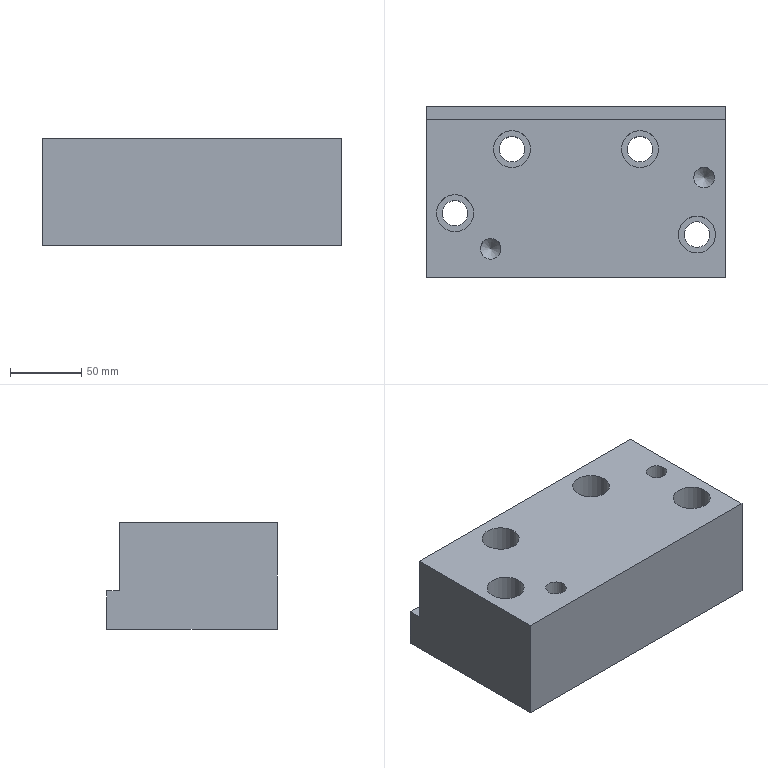Part | STEP file | lll_id550_x_t | 1 solid | 28 faces | box 210 x 120 x 75 mm | volume 1667876 mm3 | plane 12 | cylinder 12 | cone 4 | commonest cylinder face diameters 18.009 x4 26.008 x4 8.506 x2 14.506 x2
STEP:
#1=CARTESIAN_POINT('',(2294.339,-512.386,-95.));
#2=VERTEX_POINT('',#1);
#3=CARTESIAN_POINT('',(2504.339,-512.386,-95.));
#4=VERTEX_POINT('',#3);
#5=CARTESIAN_POINT('',(2648.249,-512.386,-95.));
#6=DIRECTION('',(1.,0.,0.));
#7=VECTOR('',#6,1.);
#8=LINE('',#5,#7);
#9=EDGE_CURVE('',#2,#4,#8,.T.);
#10=ORIENTED_EDGE('',*,*,#9,.T.);
#11=CARTESIAN_POINT('',(2504.339,-512.386,-20.));
#12=VERTEX_POINT('',#11);
#13=CARTESIAN_POINT('',(2504.339,-512.386,-60.));
#14=DIRECTION('',(0.,0.,-1.));
#15=VECTOR('',#14,1.);
#16=LINE('',#13,#15);
#17=EDGE_CURVE('',#12,#4,#16,.T.);
#18=ORIENTED_EDGE('',*,*,#17,.F.);
#19=CARTESIAN_POINT('',(2294.339,-512.386,-20.));
#20=VERTEX_POINT('',#19);
#21=CARTESIAN_POINT('',(-2203.001,-512.386,-20.));
#22=DIRECTION('',(-1.,0.,0.));
#23=VECTOR('',#22,1.);
#24=LINE('',#21,#23);
#25=EDGE_CURVE('',#12,#20,#24,.T.);
#26=ORIENTED_EDGE('',*,*,#25,.T.);
#27=CARTESIAN_POINT('',(2294.339,-512.386,72.5));
#28=DIRECTION('',(0.,0.,-1.));
#29=VECTOR('',#28,1.);
#30=LINE('',#27,#29);
#31=EDGE_CURVE('',#20,#2,#30,.T.);
#32=ORIENTED_EDGE('',*,*,#31,.T.);
#33=EDGE_LOOP('',(#10,#18,#26,#32));
#34=FACE_OUTER_BOUND('',#33,.T.);
#35=CARTESIAN_POINT('',(-2203.001,-512.386,-650.));
#36=DIRECTION('',(0.,1.,0.));
#37=DIRECTION('',(0.,0.,1.));
#38=AXIS2_PLACEMENT_3D('',#35,#36,#37);
#39=PLANE('',#38);
#40=ADVANCED_FACE('',(#34),#39,.F.);
#41=CARTESIAN_POINT('',(2493.344,-482.386,-95.));
#42=VERTEX_POINT('',#41);
#43=CARTESIAN_POINT('',(2484.339,-482.386,-95.));
#44=DIRECTION('',(0.,0.,1.));
#45=DIRECTION('',(1.,0.,0.));
#46=AXIS2_PLACEMENT_3D('',#43,#44,#45);
#47=CIRCLE('',#46,9.005);
#48=EDGE_CURVE('',#42,#42,#47,.T.);
#49=ORIENTED_EDGE('',*,*,#48,.T.);
#50=EDGE_LOOP('',(#49));
#51=FACE_BOUND('',#50,.T.);
#52=CARTESIAN_POINT('',(2323.344,-467.386,-95.));
#53=VERTEX_POINT('',#52);
#54=CARTESIAN_POINT('',(2314.339,-467.386,-95.));
#55=DIRECTION('',(0.,0.,1.));
#56=DIRECTION('',(1.,0.,0.));
#57=AXIS2_PLACEMENT_3D('',#54,#55,#56);
#58=CIRCLE('',#57,9.005);
#59=EDGE_CURVE('',#53,#53,#58,.T.);
#60=ORIENTED_EDGE('',*,*,#59,.T.);
#61=EDGE_LOOP('',(#60));
#62=FACE_BOUND('',#61,.T.);
#63=CARTESIAN_POINT('',(2453.344,-422.386,-95.));
#64=VERTEX_POINT('',#63);
#65=CARTESIAN_POINT('',(2444.339,-422.386,-95.));
#66=DIRECTION('',(0.,0.,1.));
#67=DIRECTION('',(1.,0.,0.));
#68=AXIS2_PLACEMENT_3D('',#65,#66,#67);
#69=CIRCLE('',#68,9.005);
#70=EDGE_CURVE('',#64,#64,#69,.T.);
#71=ORIENTED_EDGE('',*,*,#70,.T.);
#72=EDGE_LOOP('',(#71));
#73=FACE_BOUND('',#72,.T.);
#74=CARTESIAN_POINT('',(2363.344,-422.386,-95.));
#75=VERTEX_POINT('',#74);
#76=CARTESIAN_POINT('',(2354.339,-422.386,-95.));
#77=DIRECTION('',(0.,0.,1.));
#78=DIRECTION('',(1.,0.,0.));
#79=AXIS2_PLACEMENT_3D('',#76,#77,#78);
#80=CIRCLE('',#79,9.005);
#81=EDGE_CURVE('',#75,#75,#80,.T.);
#82=ORIENTED_EDGE('',*,*,#81,.T.);
#83=EDGE_LOOP('',(#82));
#84=FACE_BOUND('',#83,.T.);
#85=ORIENTED_EDGE('',*,*,#9,.F.);
#86=CARTESIAN_POINT('',(2294.339,-392.386,-95.));
#87=VERTEX_POINT('',#86);
#88=CARTESIAN_POINT('',(2294.339,-442.386,-95.));
#89=DIRECTION('',(0.,1.,0.));
#90=VECTOR('',#89,1.);
#91=LINE('',#88,#90);
#92=EDGE_CURVE('',#2,#87,#91,.T.);
#93=ORIENTED_EDGE('',*,*,#92,.T.);
#94=CARTESIAN_POINT('',(2504.339,-392.386,-95.));
#95=VERTEX_POINT('',#94);
#96=CARTESIAN_POINT('',(-2203.001,-392.386,-95.));
#97=DIRECTION('',(1.,0.,0.));
#98=VECTOR('',#97,1.);
#99=LINE('',#96,#98);
#100=EDGE_CURVE('',#87,#95,#99,.T.);
#101=ORIENTED_EDGE('',*,*,#100,.T.);
#102=CARTESIAN_POINT('',(2504.339,-268.547,-95.));
#103=DIRECTION('',(0.,-1.,0.));
#104=VECTOR('',#103,1.);
#105=LINE('',#102,#104);
#106=EDGE_CURVE('',#95,#4,#105,.T.);
#107=ORIENTED_EDGE('',*,*,#106,.T.);
#108=EDGE_LOOP('',(#85,#93,#101,#107));
#109=FACE_BOUND('',#108,.T.);
#110=CARTESIAN_POINT('',(2648.249,-268.547,-95.));
#111=DIRECTION('',(0.,0.,-1.));
#112=DIRECTION('',(1.,0.,0.));
#113=AXIS2_PLACEMENT_3D('',#110,#111,#112);
#114=PLANE('',#113);
#115=ADVANCED_FACE('',(#51,#62,#73,#84,#109),#114,.T.);
#116=CARTESIAN_POINT('',(2504.339,-401.386,-20.));
#117=VERTEX_POINT('',#116);
#118=CARTESIAN_POINT('',(2504.339,-417.386,-20.));
#119=DIRECTION('',(0.,1.,0.));
#120=VECTOR('',#119,1.);
#121=LINE('',#118,#120);
#122=EDGE_CURVE('',#12,#117,#121,.T.);
#123=ORIENTED_EDGE('',*,*,#122,.T.);
#124=CARTESIAN_POINT('',(2294.339,-401.386,-20.));
#125=VERTEX_POINT('',#124);
#126=CARTESIAN_POINT('',(-2203.001,-401.386,-20.));
#127=DIRECTION('',(1.,0.,0.));
#128=VECTOR('',#127,1.);
#129=LINE('',#126,#128);
#130=EDGE_CURVE('',#125,#117,#129,.T.);
#131=ORIENTED_EDGE('',*,*,#130,.F.);
#132=CARTESIAN_POINT('',(2294.339,-417.386,-20.));
#133=DIRECTION('',(0.,-1.,0.));
#134=VECTOR('',#133,1.);
#135=LINE('',#132,#134);
#136=EDGE_CURVE('',#125,#20,#135,.T.);
#137=ORIENTED_EDGE('',*,*,#136,.T.);
#138=ORIENTED_EDGE('',*,*,#25,.F.);
#139=EDGE_LOOP('',(#123,#131,#137,#138));
#140=FACE_BOUND('',#139,.T.);
#141=CARTESIAN_POINT('',(2346.592,-492.386,-20.));
#142=VERTEX_POINT('',#141);
#143=CARTESIAN_POINT('',(2339.339,-492.386,-20.));
#144=DIRECTION('',(0.,0.,1.));
#145=DIRECTION('',(1.,0.,0.));
#146=AXIS2_PLACEMENT_3D('',#143,#144,#145);
#147=CIRCLE('',#146,7.253);
#148=EDGE_CURVE('',#142,#142,#147,.T.);
#149=ORIENTED_EDGE('',*,*,#148,.F.);
#150=EDGE_LOOP('',(#149));
#151=FACE_BOUND('',#150,.T.);
#152=CARTESIAN_POINT('',(2496.592,-442.386,-20.));
#153=VERTEX_POINT('',#152);
#154=CARTESIAN_POINT('',(2489.339,-442.386,-20.));
#155=DIRECTION('',(0.,0.,1.));
#156=DIRECTION('',(1.,0.,0.));
#157=AXIS2_PLACEMENT_3D('',#154,#155,#156);
#158=CIRCLE('',#157,7.253);
#159=EDGE_CURVE('',#153,#153,#158,.T.);
#160=ORIENTED_EDGE('',*,*,#159,.F.);
#161=EDGE_LOOP('',(#160));
#162=FACE_BOUND('',#161,.T.);
#163=CARTESIAN_POINT('',(2471.335,-482.386,-20.));
#164=VERTEX_POINT('',#163);
#165=CARTESIAN_POINT('',(2484.339,-482.386,-20.));
#166=DIRECTION('',(0.,0.,1.));
#167=DIRECTION('',(-1.,0.,0.));
#168=AXIS2_PLACEMENT_3D('',#165,#166,#167);
#169=CIRCLE('',#168,13.004);
#170=EDGE_CURVE('',#164,#164,#169,.T.);
#171=ORIENTED_EDGE('',*,*,#170,.F.);
#172=EDGE_LOOP('',(#171));
#173=FACE_BOUND('',#172,.T.);
#174=CARTESIAN_POINT('',(2301.335,-467.386,-20.));
#175=VERTEX_POINT('',#174);
#176=CARTESIAN_POINT('',(2314.339,-467.386,-20.));
#177=DIRECTION('',(0.,0.,1.));
#178=DIRECTION('',(-1.,0.,0.));
#179=AXIS2_PLACEMENT_3D('',#176,#177,#178);
#180=CIRCLE('',#179,13.004);
#181=EDGE_CURVE('',#175,#175,#180,.T.);
#182=ORIENTED_EDGE('',*,*,#181,.F.);
#183=EDGE_LOOP('',(#182));
#184=FACE_BOUND('',#183,.T.);
#185=CARTESIAN_POINT('',(2431.335,-422.386,-20.));
#186=VERTEX_POINT('',#185);
#187=CARTESIAN_POINT('',(2444.339,-422.386,-20.));
#188=DIRECTION('',(0.,0.,1.));
#189=DIRECTION('',(-1.,0.,0.));
#190=AXIS2_PLACEMENT_3D('',#187,#188,#189);
#191=CIRCLE('',#190,13.004);
#192=EDGE_CURVE('',#186,#186,#191,.T.);
#193=ORIENTED_EDGE('',*,*,#192,.F.);
#194=EDGE_LOOP('',(#193));
#195=FACE_BOUND('',#194,.T.);
#196=CARTESIAN_POINT('',(2367.343,-422.386,-20.));
#197=VERTEX_POINT('',#196);
#198=CARTESIAN_POINT('',(2354.339,-422.386,-20.));
#199=DIRECTION('',(0.,0.,-1.));
#200=DIRECTION('',(1.,0.,0.));
#201=AXIS2_PLACEMENT_3D('',#198,#199,#200);
#202=CIRCLE('',#201,13.004);
#203=EDGE_CURVE('',#197,#197,#202,.T.);
#204=ORIENTED_EDGE('',*,*,#203,.T.);
#205=EDGE_LOOP('',(#204));
#206=FACE_BOUND('',#205,.T.);
#207=CARTESIAN_POINT('',(2402.588,-417.386,-20.));
#208=DIRECTION('',(0.,0.,-1.));
#209=DIRECTION('',(1.,0.,0.));
#210=AXIS2_PLACEMENT_3D('',#207,#208,#209);
#211=PLANE('',#210);
#212=ADVANCED_FACE('',(#140,#151,#162,#173,#184,#195,#206),#211,.F.);
#213=CARTESIAN_POINT('',(2470.086,-401.386,-44.));
#214=VERTEX_POINT('',#213);
#215=CARTESIAN_POINT('',(2474.339,-401.386,-44.));
#216=DIRECTION('',(0.,1.,0.));
#217=DIRECTION('',(-1.,0.,0.));
#218=AXIS2_PLACEMENT_3D('',#215,#216,#217);
#219=CIRCLE('',#218,4.253);
#220=EDGE_CURVE('',#214,#214,#219,.T.);
#221=ORIENTED_EDGE('',*,*,#220,.F.);
#222=EDGE_LOOP('',(#221));
#223=FACE_BOUND('',#222,.T.);
#224=CARTESIAN_POINT('',(2294.339,-401.386,-68.));
#225=VERTEX_POINT('',#224);
#226=CARTESIAN_POINT('',(2504.339,-401.386,-68.));
#227=VERTEX_POINT('',#226);
#228=CARTESIAN_POINT('',(2399.339,-401.386,-68.));
#229=DIRECTION('',(1.,0.,0.));
#230=VECTOR('',#229,1.);
#231=LINE('',#228,#230);
#232=EDGE_CURVE('',#225,#227,#231,.T.);
#233=ORIENTED_EDGE('',*,*,#232,.F.);
#234=CARTESIAN_POINT('',(2294.339,-401.386,-650.));
#235=DIRECTION('',(0.,0.,-1.));
#236=VECTOR('',#235,1.);
#237=LINE('',#234,#236);
#238=EDGE_CURVE('',#125,#225,#237,.T.);
#239=ORIENTED_EDGE('',*,*,#238,.F.);
#240=ORIENTED_EDGE('',*,*,#130,.T.);
#241=CARTESIAN_POINT('',(2504.339,-401.386,-60.));
#242=DIRECTION('',(0.,0.,1.));
#243=VECTOR('',#242,1.);
#244=LINE('',#241,#243);
#245=EDGE_CURVE('',#227,#117,#244,.T.);
#246=ORIENTED_EDGE('',*,*,#245,.F.);
#247=EDGE_LOOP('',(#233,#239,#240,#246));
#248=FACE_BOUND('',#247,.T.);
#249=CARTESIAN_POINT('',(2320.086,-401.386,-44.));
#250=VERTEX_POINT('',#249);
#251=CARTESIAN_POINT('',(2324.339,-401.386,-44.));
#252=DIRECTION('',(0.,1.,0.));
#253=DIRECTION('',(-1.,0.,0.));
#254=AXIS2_PLACEMENT_3D('',#251,#252,#253);
#255=CIRCLE('',#254,4.253);
#256=EDGE_CURVE('',#250,#250,#255,.T.);
#257=ORIENTED_EDGE('',*,*,#256,.F.);
#258=EDGE_LOOP('',(#257));
#259=FACE_BOUND('',#258,.T.);
#260=CARTESIAN_POINT('',(-2203.001,-401.386,-650.));
#261=DIRECTION('',(0.,1.,0.));
#262=DIRECTION('',(0.,0.,1.));
#263=AXIS2_PLACEMENT_3D('',#260,#261,#262);
#264=PLANE('',#263);
#265=ADVANCED_FACE('',(#223,#248,#259),#264,.T.);
#266=CARTESIAN_POINT('',(2294.339,-392.386,-68.));
#267=VERTEX_POINT('',#266);
#268=CARTESIAN_POINT('',(2294.339,-392.386,72.5));
#269=DIRECTION('',(0.,0.,-1.));
#270=VECTOR('',#269,1.);
#271=LINE('',#268,#270);
#272=EDGE_CURVE('',#267,#87,#271,.T.);
#273=ORIENTED_EDGE('',*,*,#272,.T.);
#274=ORIENTED_EDGE('',*,*,#92,.F.);
#275=ORIENTED_EDGE('',*,*,#31,.F.);
#276=ORIENTED_EDGE('',*,*,#136,.F.);
#277=ORIENTED_EDGE('',*,*,#238,.T.);
#278=CARTESIAN_POINT('',(2294.339,-432.386,-68.));
#279=DIRECTION('',(0.,1.,0.));
#280=VECTOR('',#279,1.);
#281=LINE('',#278,#280);
#282=EDGE_CURVE('',#225,#267,#281,.T.);
#283=ORIENTED_EDGE('',*,*,#282,.T.);
#284=EDGE_LOOP('',(#273,#274,#275,#276,#277,#283));
#285=FACE_OUTER_BOUND('',#284,.T.);
#286=CARTESIAN_POINT('',(2294.339,-442.386,72.5));
#287=DIRECTION('',(-1.,0.,0.));
#288=DIRECTION('',(0.,0.,-1.));
#289=AXIS2_PLACEMENT_3D('',#286,#287,#288);
#290=PLANE('',#289);
#291=ADVANCED_FACE('',(#285),#290,.T.);
#292=CARTESIAN_POINT('',(2504.339,-392.386,-68.));
#293=VERTEX_POINT('',#292);
#294=CARTESIAN_POINT('',(2504.339,-392.386,-60.));
#295=DIRECTION('',(0.,0.,1.));
#296=VECTOR('',#295,1.);
#297=LINE('',#294,#296);
#298=EDGE_CURVE('',#95,#293,#297,.T.);
#299=ORIENTED_EDGE('',*,*,#298,.F.);
#300=ORIENTED_EDGE('',*,*,#100,.F.);
#301=ORIENTED_EDGE('',*,*,#272,.F.);
#302=CARTESIAN_POINT('',(-2203.001,-392.386,-68.));
#303=DIRECTION('',(-1.,0.,0.));
#304=VECTOR('',#303,1.);
#305=LINE('',#302,#304);
#306=EDGE_CURVE('',#293,#267,#305,.T.);
#307=ORIENTED_EDGE('',*,*,#306,.F.);
#308=EDGE_LOOP('',(#299,#300,#301,#307));
#309=FACE_OUTER_BOUND('',#308,.T.);
#310=CARTESIAN_POINT('',(-2203.001,-392.386,-650.));
#311=DIRECTION('',(0.,1.,0.));
#312=DIRECTION('',(0.,0.,1.));
#313=AXIS2_PLACEMENT_3D('',#310,#311,#312);
#314=PLANE('',#313);
#315=ADVANCED_FACE('',(#309),#314,.T.);
#316=CARTESIAN_POINT('',(2504.339,-417.386,-68.));
#317=DIRECTION('',(0.,-1.,0.));
#318=VECTOR('',#317,1.);
#319=LINE('',#316,#318);
#320=EDGE_CURVE('',#293,#227,#319,.T.);
#321=ORIENTED_EDGE('',*,*,#320,.T.);
#322=ORIENTED_EDGE('',*,*,#245,.T.);
#323=ORIENTED_EDGE('',*,*,#122,.F.);
#324=ORIENTED_EDGE('',*,*,#17,.T.);
#325=ORIENTED_EDGE('',*,*,#106,.F.);
#326=ORIENTED_EDGE('',*,*,#298,.T.);
#327=EDGE_LOOP('',(#321,#322,#323,#324,#325,#326));
#328=FACE_OUTER_BOUND('',#327,.T.);
#329=CARTESIAN_POINT('',(2504.339,-417.386,-60.));
#330=DIRECTION('',(-1.,0.,0.));
#331=DIRECTION('',(0.,0.,-1.));
#332=AXIS2_PLACEMENT_3D('',#329,#330,#331);
#333=PLANE('',#332);
#334=ADVANCED_FACE('',(#328),#333,.F.);
#335=ORIENTED_EDGE('',*,*,#232,.T.);
#336=ORIENTED_EDGE('',*,*,#320,.F.);
#337=ORIENTED_EDGE('',*,*,#306,.T.);
#338=ORIENTED_EDGE('',*,*,#282,.F.);
#339=EDGE_LOOP('',(#335,#336,#337,#338));
#340=FACE_OUTER_BOUND('',#339,.T.);
#341=CARTESIAN_POINT('',(2399.339,-432.386,-68.));
#342=DIRECTION('',(0.,0.,1.));
#343=DIRECTION('',(-1.,0.,0.));
#344=AXIS2_PLACEMENT_3D('',#341,#342,#343);
#345=PLANE('',#344);
#346=ADVANCED_FACE('',(#340),#345,.T.);
#347=CARTESIAN_POINT('',(2474.339,-432.139,-48.253));
#348=VERTEX_POINT('',#347);
#349=CARTESIAN_POINT('',(2474.339,-432.139,-44.));
#350=DIRECTION('',(0.,1.,0.));
#351=DIRECTION('',(0.,0.,-1.));
#352=AXIS2_PLACEMENT_3D('',#349,#350,#351);
#353=CIRCLE('',#352,4.253);
#354=EDGE_CURVE('',#348,#348,#353,.T.);
#355=ORIENTED_EDGE('',*,*,#354,.F.);
#356=EDGE_LOOP('',(#355));
#357=FACE_BOUND('',#356,.T.);
#358=ORIENTED_EDGE('',*,*,#220,.T.);
#359=EDGE_LOOP('',(#358));
#360=FACE_BOUND('',#359,.T.);
#361=CARTESIAN_POINT('',(2474.339,-401.386,-44.));
#362=DIRECTION('',(0.,-1.,0.));
#363=DIRECTION('',(-1.,0.,0.));
#364=AXIS2_PLACEMENT_3D('',#361,#362,#363);
#365=CYLINDRICAL_SURFACE('',#364,4.253);
#366=ADVANCED_FACE('',(#357,#360),#365,.F.);
#367=CARTESIAN_POINT('',(2474.339,-436.392,-44.));
#368=VERTEX_POINT('',#367);
#369=VERTEX_LOOP('',#368);
#370=FACE_BOUND('',#369,.T.);
#371=ORIENTED_EDGE('',*,*,#354,.T.);
#372=EDGE_LOOP('',(#371));
#373=FACE_BOUND('',#372,.T.);
#374=CARTESIAN_POINT('',(2474.339,-432.139,-44.));
#375=DIRECTION('',(0.,1.,0.));
#376=DIRECTION('',(0.,0.,1.));
#377=AXIS2_PLACEMENT_3D('',#374,#375,#376);
#378=CONICAL_SURFACE('',#377,4.253,45.);
#379=ADVANCED_FACE('',(#370,#373),#378,.F.);
#380=CARTESIAN_POINT('',(2324.339,-432.139,-48.253));
#381=VERTEX_POINT('',#380);
#382=CARTESIAN_POINT('',(2324.339,-432.139,-44.));
#383=DIRECTION('',(0.,1.,0.));
#384=DIRECTION('',(0.,0.,-1.));
#385=AXIS2_PLACEMENT_3D('',#382,#383,#384);
#386=CIRCLE('',#385,4.253);
#387=EDGE_CURVE('',#381,#381,#386,.T.);
#388=ORIENTED_EDGE('',*,*,#387,.F.);
#389=EDGE_LOOP('',(#388));
#390=FACE_BOUND('',#389,.T.);
#391=ORIENTED_EDGE('',*,*,#256,.T.);
#392=EDGE_LOOP('',(#391));
#393=FACE_BOUND('',#392,.T.);
#394=CARTESIAN_POINT('',(2324.339,-401.386,-44.));
#395=DIRECTION('',(0.,-1.,0.));
#396=DIRECTION('',(-1.,0.,0.));
#397=AXIS2_PLACEMENT_3D('',#394,#395,#396);
#398=CYLINDRICAL_SURFACE('',#397,4.253);
#399=ADVANCED_FACE('',(#390,#393),#398,.F.);
#400=CARTESIAN_POINT('',(2324.339,-436.392,-44.));
#401=VERTEX_POINT('',#400);
#402=VERTEX_LOOP('',#401);
#403=FACE_BOUND('',#402,.T.);
#404=ORIENTED_EDGE('',*,*,#387,.T.);
#405=EDGE_LOOP('',(#404));
#406=FACE_BOUND('',#405,.T.);
#407=CARTESIAN_POINT('',(2324.339,-432.139,-44.));
#408=DIRECTION('',(0.,1.,0.));
#409=DIRECTION('',(0.,0.,1.));
#410=AXIS2_PLACEMENT_3D('',#407,#408,#409);
#411=CONICAL_SURFACE('',#410,4.253,45.);
#412=ADVANCED_FACE('',(#403,#406),#411,.F.);
#413=ORIENTED_EDGE('',*,*,#48,.F.);
#414=EDGE_LOOP('',(#413));
#415=FACE_BOUND('',#414,.T.);
#416=CARTESIAN_POINT('',(2493.344,-482.386,-55.));
#417=VERTEX_POINT('',#416);
#418=CARTESIAN_POINT('',(2484.339,-482.386,-55.));
#419=DIRECTION('',(0.,0.,1.));
#420=DIRECTION('',(1.,0.,0.));
#421=AXIS2_PLACEMENT_3D('',#418,#419,#420);
#422=CIRCLE('',#421,9.005);
#423=EDGE_CURVE('',#417,#417,#422,.T.);
#424=ORIENTED_EDGE('',*,*,#423,.T.);
#425=EDGE_LOOP('',(#424));
#426=FACE_BOUND('',#425,.T.);
#427=CARTESIAN_POINT('',(2484.339,-482.386,-18.));
#428=DIRECTION('',(0.,0.,-1.));
#429=DIRECTION('',(-1.,0.,0.));
#430=AXIS2_PLACEMENT_3D('',#427,#428,#429);
#431=CYLINDRICAL_SURFACE('',#430,9.005);
#432=ADVANCED_FACE('',(#415,#426),#431,.F.);
#433=ORIENTED_EDGE('',*,*,#423,.F.);
#434=EDGE_LOOP('',(#433));
#435=FACE_BOUND('',#434,.T.);
#436=CARTESIAN_POINT('',(2471.335,-482.386,-55.));
#437=VERTEX_POINT('',#436);
#438=CARTESIAN_POINT('',(2484.339,-482.386,-55.));
#439=DIRECTION('',(0.,0.,1.));
#440=DIRECTION('',(-1.,0.,0.));
#441=AXIS2_PLACEMENT_3D('',#438,#439,#440);
#442=CIRCLE('',#441,13.004);
#443=EDGE_CURVE('',#437,#437,#442,.T.);
#444=ORIENTED_EDGE('',*,*,#443,.T.);
#445=EDGE_LOOP('',(#444));
#446=FACE_BOUND('',#445,.T.);
#447=CARTESIAN_POINT('',(2484.339,-482.386,-55.));
#448=DIRECTION('',(0.,0.,-1.));
#449=DIRECTION('',(1.,0.,0.));
#450=AXIS2_PLACEMENT_3D('',#447,#448,#449);
#451=PLANE('',#450);
#452=ADVANCED_FACE('',(#435,#446),#451,.F.);
#453=ORIENTED_EDGE('',*,*,#443,.F.);
#454=EDGE_LOOP('',(#453));
#455=FACE_BOUND('',#454,.T.);
#456=ORIENTED_EDGE('',*,*,#170,.T.);
#457=EDGE_LOOP('',(#456));
#458=FACE_BOUND('',#457,.T.);
#459=CARTESIAN_POINT('',(2484.339,-482.386,-20.));
#460=DIRECTION('',(0.,0.,-1.));
#461=DIRECTION('',(-1.,0.,0.));
#462=AXIS2_PLACEMENT_3D('',#459,#460,#461);
#463=CYLINDRICAL_SURFACE('',#462,13.004);
#464=ADVANCED_FACE('',(#455,#458),#463,.F.);
#465=ORIENTED_EDGE('',*,*,#59,.F.);
#466=EDGE_LOOP('',(#465));
#467=FACE_BOUND('',#466,.T.);
#468=CARTESIAN_POINT('',(2323.344,-467.386,-55.));
#469=VERTEX_POINT('',#468);
#470=CARTESIAN_POINT('',(2314.339,-467.386,-55.));
#471=DIRECTION('',(0.,0.,1.));
#472=DIRECTION('',(1.,0.,0.));
#473=AXIS2_PLACEMENT_3D('',#470,#471,#472);
#474=CIRCLE('',#473,9.005);
#475=EDGE_CURVE('',#469,#469,#474,.T.);
#476=ORIENTED_EDGE('',*,*,#475,.T.);
#477=EDGE_LOOP('',(#476));
#478=FACE_BOUND('',#477,.T.);
#479=CARTESIAN_POINT('',(2314.339,-467.386,-18.));
#480=DIRECTION('',(0.,0.,-1.));
#481=DIRECTION('',(-1.,0.,0.));
#482=AXIS2_PLACEMENT_3D('',#479,#480,#481);
#483=CYLINDRICAL_SURFACE('',#482,9.005);
#484=ADVANCED_FACE('',(#467,#478),#483,.F.);
#485=ORIENTED_EDGE('',*,*,#475,.F.);
#486=EDGE_LOOP('',(#485));
#487=FACE_BOUND('',#486,.T.);
#488=CARTESIAN_POINT('',(2301.335,-467.386,-55.));
#489=VERTEX_POINT('',#488);
#490=CARTESIAN_POINT('',(2314.339,-467.386,-55.));
#491=DIRECTION('',(0.,0.,1.));
#492=DIRECTION('',(-1.,0.,0.));
#493=AXIS2_PLACEMENT_3D('',#490,#491,#492);
#494=CIRCLE('',#493,13.004);
#495=EDGE_CURVE('',#489,#489,#494,.T.);
#496=ORIENTED_EDGE('',*,*,#495,.T.);
#497=EDGE_LOOP('',(#496));
#498=FACE_BOUND('',#497,.T.);
#499=CARTESIAN_POINT('',(2314.339,-467.386,-55.));
#500=DIRECTION('',(0.,0.,-1.));
#501=DIRECTION('',(1.,0.,0.));
#502=AXIS2_PLACEMENT_3D('',#499,#500,#501);
#503=PLANE('',#502);
#504=ADVANCED_FACE('',(#487,#498),#503,.F.);
#505=ORIENTED_EDGE('',*,*,#495,.F.);
#506=EDGE_LOOP('',(#505));
#507=FACE_BOUND('',#506,.T.);
#508=ORIENTED_EDGE('',*,*,#181,.T.);
#509=EDGE_LOOP('',(#508));
#510=FACE_BOUND('',#509,.T.);
#511=CARTESIAN_POINT('',(2314.339,-467.386,-20.));
#512=DIRECTION('',(0.,0.,-1.));
#513=DIRECTION('',(-1.,0.,0.));
#514=AXIS2_PLACEMENT_3D('',#511,#512,#513);
#515=CYLINDRICAL_SURFACE('',#514,13.004);
#516=ADVANCED_FACE('',(#507,#510),#515,.F.);
#517=ORIENTED_EDGE('',*,*,#70,.F.);
#518=EDGE_LOOP('',(#517));
#519=FACE_BOUND('',#518,.T.);
#520=CARTESIAN_POINT('',(2453.344,-422.386,-55.));
#521=VERTEX_POINT('',#520);
#522=CARTESIAN_POINT('',(2444.339,-422.386,-55.));
#523=DIRECTION('',(0.,0.,1.));
#524=DIRECTION('',(1.,0.,0.));
#525=AXIS2_PLACEMENT_3D('',#522,#523,#524);
#526=CIRCLE('',#525,9.005);
#527=EDGE_CURVE('',#521,#521,#526,.T.);
#528=ORIENTED_EDGE('',*,*,#527,.T.);
#529=EDGE_LOOP('',(#528));
#530=FACE_BOUND('',#529,.T.);
#531=CARTESIAN_POINT('',(2444.339,-422.386,-18.));
#532=DIRECTION('',(0.,0.,-1.));
#533=DIRECTION('',(-1.,0.,0.));
#534=AXIS2_PLACEMENT_3D('',#531,#532,#533);
#535=CYLINDRICAL_SURFACE('',#534,9.005);
#536=ADVANCED_FACE('',(#519,#530),#535,.F.);
#537=ORIENTED_EDGE('',*,*,#527,.F.);
#538=EDGE_LOOP('',(#537));
#539=FACE_BOUND('',#538,.T.);
#540=CARTESIAN_POINT('',(2431.335,-422.386,-55.));
#541=VERTEX_POINT('',#540);
#542=CARTESIAN_POINT('',(2444.339,-422.386,-55.));
#543=DIRECTION('',(0.,0.,1.));
#544=DIRECTION('',(-1.,0.,0.));
#545=AXIS2_PLACEMENT_3D('',#542,#543,#544);
#546=CIRCLE('',#545,13.004);
#547=EDGE_CURVE('',#541,#541,#546,.T.);
#548=ORIENTED_EDGE('',*,*,#547,.T.);
#549=EDGE_LOOP('',(#548));
#550=FACE_BOUND('',#549,.T.);
#551=CARTESIAN_POINT('',(2444.339,-422.386,-55.));
#552=DIRECTION('',(0.,0.,-1.));
#553=DIRECTION('',(1.,0.,0.));
#554=AXIS2_PLACEMENT_3D('',#551,#552,#553);
#555=PLANE('',#554);
#556=ADVANCED_FACE('',(#539,#550),#555,.F.);
#557=ORIENTED_EDGE('',*,*,#547,.F.);
#558=EDGE_LOOP('',(#557));
#559=FACE_BOUND('',#558,.T.);
#560=ORIENTED_EDGE('',*,*,#192,.T.);
#561=EDGE_LOOP('',(#560));
#562=FACE_BOUND('',#561,.T.);
#563=CARTESIAN_POINT('',(2444.339,-422.386,-20.));
#564=DIRECTION('',(0.,0.,-1.));
#565=DIRECTION('',(-1.,0.,0.));
#566=AXIS2_PLACEMENT_3D('',#563,#564,#565);
#567=CYLINDRICAL_SURFACE('',#566,13.004);
#568=ADVANCED_FACE('',(#559,#562),#567,.F.);
#569=ORIENTED_EDGE('',*,*,#81,.F.);
#570=EDGE_LOOP('',(#569));
#571=FACE_BOUND('',#570,.T.);
#572=CARTESIAN_POINT('',(2345.335,-422.386,-55.));
#573=VERTEX_POINT('',#572);
#574=CARTESIAN_POINT('',(2354.339,-422.386,-55.));
#575=DIRECTION('',(0.,0.,-1.));
#576=DIRECTION('',(-1.,0.,0.));
#577=AXIS2_PLACEMENT_3D('',#574,#575,#576);
#578=CIRCLE('',#577,9.005);
#579=EDGE_CURVE('',#573,#573,#578,.T.);
#580=ORIENTED_EDGE('',*,*,#579,.F.);
#581=EDGE_LOOP('',(#580));
#582=FACE_BOUND('',#581,.T.);
#583=CARTESIAN_POINT('',(2354.339,-422.386,-18.));
#584=DIRECTION('',(0.,0.,-1.));
#585=DIRECTION('',(1.,0.,0.));
#586=AXIS2_PLACEMENT_3D('',#583,#584,#585);
#587=CYLINDRICAL_SURFACE('',#586,9.005);
#588=ADVANCED_FACE('',(#571,#582),#587,.F.);
#589=ORIENTED_EDGE('',*,*,#579,.T.);
#590=EDGE_LOOP('',(#589));
#591=FACE_BOUND('',#590,.T.);
#592=CARTESIAN_POINT('',(2367.343,-422.386,-55.));
#593=VERTEX_POINT('',#592);
#594=CARTESIAN_POINT('',(2354.339,-422.386,-55.));
#595=DIRECTION('',(0.,0.,-1.));
#596=DIRECTION('',(1.,0.,0.));
#597=AXIS2_PLACEMENT_3D('',#594,#595,#596);
#598=CIRCLE('',#597,13.004);
#599=EDGE_CURVE('',#593,#593,#598,.T.);
#600=ORIENTED_EDGE('',*,*,#599,.F.);
#601=EDGE_LOOP('',(#600));
#602=FACE_BOUND('',#601,.T.);
#603=CARTESIAN_POINT('',(2354.339,-422.386,-55.));
#604=DIRECTION('',(0.,0.,-1.));
#605=DIRECTION('',(-1.,0.,0.));
#606=AXIS2_PLACEMENT_3D('',#603,#604,#605);
#607=PLANE('',#606);
#608=ADVANCED_FACE('',(#591,#602),#607,.F.);
#609=ORIENTED_EDGE('',*,*,#599,.T.);
#610=EDGE_LOOP('',(#609));
#611=FACE_BOUND('',#610,.T.);
#612=ORIENTED_EDGE('',*,*,#203,.F.);
#613=EDGE_LOOP('',(#612));
#614=FACE_BOUND('',#613,.T.);
#615=CARTESIAN_POINT('',(2354.339,-422.386,-20.));
#616=DIRECTION('',(0.,0.,-1.));
#617=DIRECTION('',(1.,0.,0.));
#618=AXIS2_PLACEMENT_3D('',#615,#616,#617);
#619=CYLINDRICAL_SURFACE('',#618,13.004);
#620=ADVANCED_FACE('',(#611,#614),#619,.F.);
#621=CARTESIAN_POINT('',(2496.592,-442.386,-55.753));
#622=VERTEX_POINT('',#621);
#623=CARTESIAN_POINT('',(2489.339,-442.386,-55.753));
#624=DIRECTION('',(0.,0.,1.));
#625=DIRECTION('',(1.,0.,0.));
#626=AXIS2_PLACEMENT_3D('',#623,#624,#625);
#627=CIRCLE('',#626,7.253);
#628=EDGE_CURVE('',#622,#622,#627,.T.);
#629=ORIENTED_EDGE('',*,*,#628,.F.);
#630=EDGE_LOOP('',(#629));
#631=FACE_BOUND('',#630,.T.);
#632=ORIENTED_EDGE('',*,*,#159,.T.);
#633=EDGE_LOOP('',(#632));
#634=FACE_BOUND('',#633,.T.);
#635=CARTESIAN_POINT('',(2489.339,-442.386,-18.));
#636=DIRECTION('',(0.,0.,-1.));
#637=DIRECTION('',(-1.,0.,0.));
#638=AXIS2_PLACEMENT_3D('',#635,#636,#637);
#639=CYLINDRICAL_SURFACE('',#638,7.253);
#640=ADVANCED_FACE('',(#631,#634),#639,.F.);
#641=CARTESIAN_POINT('',(2489.339,-442.386,-63.006));
#642=VERTEX_POINT('',#641);
#643=VERTEX_LOOP('',#642);
#644=FACE_BOUND('',#643,.T.);
#645=ORIENTED_EDGE('',*,*,#628,.T.);
#646=EDGE_LOOP('',(#645));
#647=FACE_BOUND('',#646,.T.);
#648=CARTESIAN_POINT('',(2489.339,-442.386,-55.753));
#649=DIRECTION('',(0.,0.,1.));
#650=DIRECTION('',(-1.,0.,0.));
#651=AXIS2_PLACEMENT_3D('',#648,#649,#650);
#652=CONICAL_SURFACE('',#651,7.253,45.);
#653=ADVANCED_FACE('',(#644,#647),#652,.F.);
#654=CARTESIAN_POINT('',(2332.086,-492.386,-55.753));
#655=VERTEX_POINT('',#654);
#656=CARTESIAN_POINT('',(2339.339,-492.386,-55.753));
#657=DIRECTION('',(0.,0.,-1.));
#658=DIRECTION('',(-1.,0.,0.));
#659=AXIS2_PLACEMENT_3D('',#656,#657,#658);
#660=CIRCLE('',#659,7.253);
#661=EDGE_CURVE('',#655,#655,#660,.T.);
#662=ORIENTED_EDGE('',*,*,#661,.T.);
#663=EDGE_LOOP('',(#662));
#664=FACE_BOUND('',#663,.T.);
#665=ORIENTED_EDGE('',*,*,#148,.T.);
#666=EDGE_LOOP('',(#665));
#667=FACE_BOUND('',#666,.T.);
#668=CARTESIAN_POINT('',(2339.339,-492.386,-18.));
#669=DIRECTION('',(0.,0.,-1.));
#670=DIRECTION('',(1.,0.,0.));
#671=AXIS2_PLACEMENT_3D('',#668,#669,#670);
#672=CYLINDRICAL_SURFACE('',#671,7.253);
#673=ADVANCED_FACE('',(#664,#667),#672,.F.);
#674=CARTESIAN_POINT('',(2339.339,-492.386,-63.006));
#675=VERTEX_POINT('',#674);
#676=VERTEX_LOOP('',#675);
#677=FACE_BOUND('',#676,.T.);
#678=ORIENTED_EDGE('',*,*,#661,.F.);
#679=EDGE_LOOP('',(#678));
#680=FACE_BOUND('',#679,.T.);
#681=CARTESIAN_POINT('',(2339.339,-492.386,-55.753));
#682=DIRECTION('',(0.,0.,1.));
#683=DIRECTION('',(1.,0.,0.));
#684=AXIS2_PLACEMENT_3D('',#681,#682,#683);
#685=CONICAL_SURFACE('',#684,7.253,45.);
#686=ADVANCED_FACE('',(#677,#680),#685,.F.);
#687=CLOSED_SHELL('',(#40,#115,#212,#265,#291,#315,#334,#346,#366,#379,#399,#412,#432,#452,#464,#484,#504,#516,#536,#556,#568,#588,#608,#620,#640,#653,#673,#686));
#688=MANIFOLD_SOLID_BREP('',#687);
#689=(LENGTH_UNIT()NAMED_UNIT(*)SI_UNIT(.MILLI.,.METRE.));
#690=UNCERTAINTY_MEASURE_WITH_UNIT(LENGTH_MEASURE(0.00002),#689,'','');
#691=(NAMED_UNIT(*)PLANE_ANGLE_UNIT()SI_UNIT($,.RADIAN.));
#692=PLANE_ANGLE_MEASURE_WITH_UNIT(PLANE_ANGLE_MEASURE(0.01745),#691);
#693=DIMENSIONAL_EXPONENTS(0.,0.,0.,0.,0.,0.,0.);
#694=(CONVERSION_BASED_UNIT('DEGREE',#692)NAMED_UNIT(#693)PLANE_ANGLE_UNIT());
#695=(NAMED_UNIT(*)SI_UNIT($,.STERADIAN.)SOLID_ANGLE_UNIT());
#696=(GEOMETRIC_REPRESENTATION_CONTEXT(3)GLOBAL_UNCERTAINTY_ASSIGNED_CONTEXT((#690))GLOBAL_UNIT_ASSIGNED_CONTEXT((#689,#694,#695))REPRESENTATION_CONTEXT('',''));
#697=ADVANCED_BREP_SHAPE_REPRESENTATION('',(#688),#696);